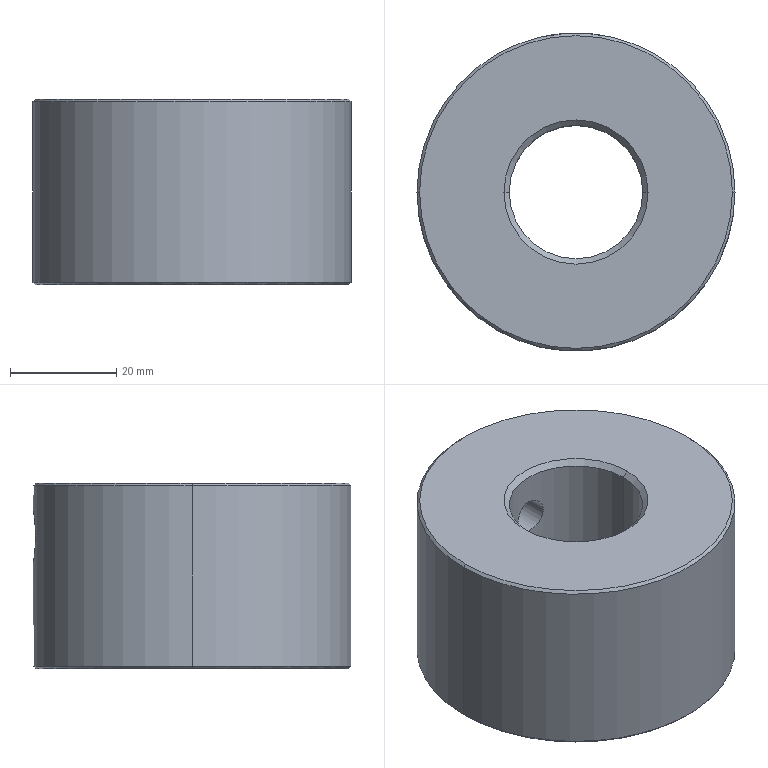Part | NX | 1 solid | 19 faces | box 60 x 60 x 35 mm | volume 80516 mm3 | cone 8 | cylinder 8 | plane 3 | commonest cylinder face diameters 6.8 x2 10 x2 25.2 x2 60 x2
STEP:
#1=CARTESIAN_POINT('',(29.5,0.,-5.));
#2=VERTEX_POINT('',#1);
#3=CARTESIAN_POINT('',(-29.5,0.,-5.));
#4=VERTEX_POINT('',#3);
#5=CARTESIAN_POINT('',(0.,0.,-5.));
#6=DIRECTION('',(0.,0.,1.));
#7=DIRECTION('',(1.,0.,0.));
#8=AXIS2_PLACEMENT_3D('',#5,#6,#7);
#9=CIRCLE('',#8,29.5);
#10=EDGE_CURVE('',#2,#4,#9,.T.);
#11=ORIENTED_EDGE('',*,*,#10,.F.);
#12=CARTESIAN_POINT('',(0.,0.,-5.));
#13=DIRECTION('',(0.,0.,1.));
#14=DIRECTION('',(1.,0.,0.));
#15=AXIS2_PLACEMENT_3D('',#12,#13,#14);
#16=CIRCLE('',#15,29.5);
#17=EDGE_CURVE('',#4,#2,#16,.T.);
#18=ORIENTED_EDGE('',*,*,#17,.F.);
#19=EDGE_LOOP('',(#11,#18));
#20=FACE_BOUND('',#19,.T.);
#21=CARTESIAN_POINT('',(13.6,0.,-5.));
#22=VERTEX_POINT('',#21);
#23=CARTESIAN_POINT('',(-13.6,0.,-5.));
#24=VERTEX_POINT('',#23);
#25=CARTESIAN_POINT('',(0.,0.,-5.));
#26=DIRECTION('',(0.,0.,1.));
#27=DIRECTION('',(1.,0.,0.));
#28=AXIS2_PLACEMENT_3D('',#25,#26,#27);
#29=CIRCLE('',#28,13.6);
#30=EDGE_CURVE('',#22,#24,#29,.T.);
#31=ORIENTED_EDGE('',*,*,#30,.T.);
#32=CARTESIAN_POINT('',(0.,0.,-5.));
#33=DIRECTION('',(0.,0.,1.));
#34=DIRECTION('',(1.,0.,0.));
#35=AXIS2_PLACEMENT_3D('',#32,#33,#34);
#36=CIRCLE('',#35,13.6);
#37=EDGE_CURVE('',#24,#22,#36,.T.);
#38=ORIENTED_EDGE('',*,*,#37,.T.);
#39=EDGE_LOOP('',(#31,#38));
#40=FACE_BOUND('',#39,.T.);
#41=CARTESIAN_POINT('',(0.,0.,-5.));
#42=DIRECTION('',(0.,0.,1.));
#43=DIRECTION('',(1.,0.,0.));
#44=AXIS2_PLACEMENT_3D('',#41,#42,#43);
#45=PLANE('',#44);
#46=ADVANCED_FACE('',(#20,#40),#45,.F.);
#47=CARTESIAN_POINT('',(12.6,0.,29.));
#48=VERTEX_POINT('',#47);
#49=CARTESIAN_POINT('',(-12.6,0.,29.));
#50=VERTEX_POINT('',#49);
#51=CARTESIAN_POINT('',(0.,0.,29.));
#52=DIRECTION('',(0.,0.,1.));
#53=DIRECTION('',(1.,0.,0.));
#54=AXIS2_PLACEMENT_3D('',#51,#52,#53);
#55=CIRCLE('',#54,12.6);
#56=EDGE_CURVE('',#48,#50,#55,.T.);
#57=ORIENTED_EDGE('',*,*,#56,.F.);
#58=CARTESIAN_POINT('',(13.6,0.,30.));
#59=VERTEX_POINT('',#58);
#60=CARTESIAN_POINT('',(13.1,0.,29.5));
#61=DIRECTION('',(0.7071,0.,0.7071));
#62=VECTOR('',#61,1000.);
#63=LINE('',#60,#62);
#64=EDGE_CURVE('',#48,#59,#63,.T.);
#65=ORIENTED_EDGE('',*,*,#64,.T.);
#66=CARTESIAN_POINT('',(-13.6,0.,30.));
#67=VERTEX_POINT('',#66);
#68=CARTESIAN_POINT('',(0.,0.,30.));
#69=DIRECTION('',(0.,0.,1.));
#70=DIRECTION('',(1.,0.,0.));
#71=AXIS2_PLACEMENT_3D('',#68,#69,#70);
#72=CIRCLE('',#71,13.6);
#73=EDGE_CURVE('',#59,#67,#72,.T.);
#74=ORIENTED_EDGE('',*,*,#73,.T.);
#75=CARTESIAN_POINT('',(-13.1,0.,29.5));
#76=DIRECTION('',(-0.7071,0.,0.7071));
#77=VECTOR('',#76,1000.);
#78=LINE('',#75,#77);
#79=EDGE_CURVE('',#50,#67,#78,.T.);
#80=ORIENTED_EDGE('',*,*,#79,.F.);
#81=EDGE_LOOP('',(#57,#65,#74,#80));
#82=FACE_BOUND('',#81,.T.);
#83=CARTESIAN_POINT('',(0.,0.,29.5));
#84=DIRECTION('',(0.,0.,1.));
#85=DIRECTION('',(1.,0.,0.));
#86=AXIS2_PLACEMENT_3D('',#83,#84,#85);
#87=CONICAL_SURFACE('',#86,13.1,0.7854);
#88=ADVANCED_FACE('',(#82),#87,.F.);
#89=CARTESIAN_POINT('',(-30.,0.,29.5));
#90=VERTEX_POINT('',#89);
#91=CARTESIAN_POINT('',(30.,0.,29.5));
#92=VERTEX_POINT('',#91);
#93=CARTESIAN_POINT('',(0.,0.,29.5));
#94=DIRECTION('',(0.,0.,-1.));
#95=DIRECTION('',(-1.,0.,0.));
#96=AXIS2_PLACEMENT_3D('',#93,#94,#95);
#97=CIRCLE('',#96,30.);
#98=EDGE_CURVE('',#90,#92,#97,.T.);
#99=ORIENTED_EDGE('',*,*,#98,.T.);
#100=CARTESIAN_POINT('',(30.,0.,-4.5));
#101=VERTEX_POINT('',#100);
#102=CARTESIAN_POINT('',(30.,0.,0.));
#103=DIRECTION('',(0.,0.,1.));
#104=VECTOR('',#103,1000.);
#105=LINE('',#102,#104);
#106=EDGE_CURVE('',#101,#92,#105,.T.);
#107=ORIENTED_EDGE('',*,*,#106,.F.);
#108=CARTESIAN_POINT('',(-30.,0.,-4.5));
#109=VERTEX_POINT('',#108);
#110=CARTESIAN_POINT('',(0.,0.,-4.5));
#111=DIRECTION('',(0.,0.,1.));
#112=DIRECTION('',(1.,0.,0.));
#113=AXIS2_PLACEMENT_3D('',#110,#111,#112);
#114=CIRCLE('',#113,30.);
#115=EDGE_CURVE('',#101,#109,#114,.T.);
#116=ORIENTED_EDGE('',*,*,#115,.T.);
#117=CARTESIAN_POINT('',(-30.,0.,0.));
#118=DIRECTION('',(0.,0.,1.));
#119=VECTOR('',#118,1000.);
#120=LINE('',#117,#119);
#121=EDGE_CURVE('',#109,#90,#120,.T.);
#122=ORIENTED_EDGE('',*,*,#121,.T.);
#123=EDGE_LOOP('',(#99,#107,#116,#122));
#124=FACE_BOUND('',#123,.T.);
#125=CARTESIAN_POINT('',(5.,29.58,20.));
#126=VERTEX_POINT('',#125);
#127=CARTESIAN_POINT('',(-5.,29.58,20.));
#128=VERTEX_POINT('',#127);
#129=CARTESIAN_POINT('',(-5.,29.58,20.));
#130=CARTESIAN_POINT('',(-5.,29.58,18.675));
#131=CARTESIAN_POINT('',(-3.919,29.792,16.092));
#132=CARTESIAN_POINT('',(0.0004669,30.104,14.454));
#133=CARTESIAN_POINT('',(3.917,29.792,16.091));
#134=CARTESIAN_POINT('',(5.,29.58,18.673));
#135=CARTESIAN_POINT('',(5.,29.58,20.));
#136=B_SPLINE_CURVE_WITH_KNOTS('',3,(#129,#130,#131,#132,#133,#134,#135),.UNSPECIFIED.,.F.,.F.,(4,1,1,1,4),(0.,0.25,0.5,0.75,1.),.UNSPECIFIED.);
#137=EDGE_CURVE('',#126,#128,#136,.F.);
#138=ORIENTED_EDGE('',*,*,#137,.F.);
#139=CARTESIAN_POINT('',(5.,29.58,20.));
#140=CARTESIAN_POINT('',(5.,29.58,21.269));
#141=CARTESIAN_POINT('',(3.919,29.792,23.936));
#142=CARTESIAN_POINT('',(0.00008607,30.104,25.533));
#143=CARTESIAN_POINT('',(-3.919,29.792,23.934));
#144=CARTESIAN_POINT('',(-5.,29.58,21.273));
#145=CARTESIAN_POINT('',(-5.,29.58,20.));
#146=B_SPLINE_CURVE_WITH_KNOTS('',3,(#139,#140,#141,#142,#143,#144,#145),.UNSPECIFIED.,.F.,.F.,(4,1,1,1,4),(0.,0.25,0.5,0.75,1.),.UNSPECIFIED.);
#147=EDGE_CURVE('',#128,#126,#146,.F.);
#148=ORIENTED_EDGE('',*,*,#147,.F.);
#149=EDGE_LOOP('',(#138,#148));
#150=FACE_BOUND('',#149,.T.);
#151=CARTESIAN_POINT('',(0.,0.,0.));
#152=DIRECTION('',(0.,0.,1.));
#153=DIRECTION('',(1.,0.,0.));
#154=AXIS2_PLACEMENT_3D('',#151,#152,#153);
#155=CYLINDRICAL_SURFACE('',#154,30.);
#156=ADVANCED_FACE('',(#124,#150),#155,.T.);
#157=CARTESIAN_POINT('',(29.5,0.,30.));
#158=VERTEX_POINT('',#157);
#159=CARTESIAN_POINT('',(-29.5,0.,30.));
#160=VERTEX_POINT('',#159);
#161=CARTESIAN_POINT('',(0.,0.,30.));
#162=DIRECTION('',(0.,0.,-1.));
#163=DIRECTION('',(-1.,0.,0.));
#164=AXIS2_PLACEMENT_3D('',#161,#162,#163);
#165=CIRCLE('',#164,29.5);
#166=EDGE_CURVE('',#158,#160,#165,.T.);
#167=ORIENTED_EDGE('',*,*,#166,.F.);
#168=CARTESIAN_POINT('',(0.,0.,30.));
#169=DIRECTION('',(0.,0.,-1.));
#170=DIRECTION('',(-1.,0.,0.));
#171=AXIS2_PLACEMENT_3D('',#168,#169,#170);
#172=CIRCLE('',#171,29.5);
#173=EDGE_CURVE('',#160,#158,#172,.T.);
#174=ORIENTED_EDGE('',*,*,#173,.F.);
#175=EDGE_LOOP('',(#167,#174));
#176=FACE_BOUND('',#175,.T.);
#177=CARTESIAN_POINT('',(0.,0.,30.));
#178=DIRECTION('',(0.,0.,1.));
#179=DIRECTION('',(1.,0.,0.));
#180=AXIS2_PLACEMENT_3D('',#177,#178,#179);
#181=CIRCLE('',#180,13.6);
#182=EDGE_CURVE('',#67,#59,#181,.T.);
#183=ORIENTED_EDGE('',*,*,#182,.F.);
#184=ORIENTED_EDGE('',*,*,#73,.F.);
#185=EDGE_LOOP('',(#183,#184));
#186=FACE_BOUND('',#185,.T.);
#187=CARTESIAN_POINT('',(0.,0.,30.));
#188=DIRECTION('',(0.,0.,1.));
#189=DIRECTION('',(1.,0.,0.));
#190=AXIS2_PLACEMENT_3D('',#187,#188,#189);
#191=PLANE('',#190);
#192=ADVANCED_FACE('',(#176,#186),#191,.T.);
#193=ORIENTED_EDGE('',*,*,#115,.F.);
#194=CARTESIAN_POINT('',(30.,0.,-4.5));
#195=DIRECTION('',(0.7071,0.,0.7071));
#196=VECTOR('',#195,1000.);
#197=LINE('',#194,#196);
#198=EDGE_CURVE('',#2,#101,#197,.T.);
#199=ORIENTED_EDGE('',*,*,#198,.F.);
#200=ORIENTED_EDGE('',*,*,#10,.T.);
#201=CARTESIAN_POINT('',(-30.,0.,-4.5));
#202=DIRECTION('',(-0.7071,0.,0.7071));
#203=VECTOR('',#202,1000.);
#204=LINE('',#201,#203);
#205=EDGE_CURVE('',#4,#109,#204,.T.);
#206=ORIENTED_EDGE('',*,*,#205,.T.);
#207=EDGE_LOOP('',(#193,#199,#200,#206));
#208=FACE_BOUND('',#207,.T.);
#209=CARTESIAN_POINT('',(0.,0.,-4.5));
#210=DIRECTION('',(0.,0.,1.));
#211=DIRECTION('',(1.,0.,0.));
#212=AXIS2_PLACEMENT_3D('',#209,#210,#211);
#213=CONICAL_SURFACE('',#212,30.,0.7854);
#214=ADVANCED_FACE('',(#208),#213,.T.);
#215=ORIENTED_EDGE('',*,*,#56,.T.);
#216=CARTESIAN_POINT('',(-12.6,0.,-4.));
#217=VERTEX_POINT('',#216);
#218=CARTESIAN_POINT('',(-12.6,0.,0.));
#219=DIRECTION('',(0.,0.,1.));
#220=VECTOR('',#219,1000.);
#221=LINE('',#218,#220);
#222=EDGE_CURVE('',#50,#217,#221,.F.);
#223=ORIENTED_EDGE('',*,*,#222,.T.);
#224=CARTESIAN_POINT('',(12.6,0.,-4.));
#225=VERTEX_POINT('',#224);
#226=CARTESIAN_POINT('',(0.,0.,-4.));
#227=DIRECTION('',(0.,0.,1.));
#228=DIRECTION('',(1.,0.,0.));
#229=AXIS2_PLACEMENT_3D('',#226,#227,#228);
#230=CIRCLE('',#229,12.6);
#231=EDGE_CURVE('',#225,#217,#230,.T.);
#232=ORIENTED_EDGE('',*,*,#231,.F.);
#233=CARTESIAN_POINT('',(12.6,0.,0.));
#234=DIRECTION('',(0.,0.,1.));
#235=VECTOR('',#234,1000.);
#236=LINE('',#233,#235);
#237=EDGE_CURVE('',#48,#225,#236,.F.);
#238=ORIENTED_EDGE('',*,*,#237,.F.);
#239=EDGE_LOOP('',(#215,#223,#232,#238));
#240=FACE_BOUND('',#239,.T.);
#241=CARTESIAN_POINT('',(-3.4,12.133,20.));
#242=VERTEX_POINT('',#241);
#243=CARTESIAN_POINT('',(3.4,12.133,20.));
#244=VERTEX_POINT('',#243);
#245=CARTESIAN_POINT('',(-3.4,12.133,20.));
#246=CARTESIAN_POINT('',(-3.4,12.133,20.9));
#247=CARTESIAN_POINT('',(-2.664,12.371,22.659));
#248=CARTESIAN_POINT('',(-0.00003224,12.715,23.771));
#249=CARTESIAN_POINT('',(2.664,12.371,22.658));
#250=CARTESIAN_POINT('',(3.4,12.133,20.901));
#251=CARTESIAN_POINT('',(3.4,12.133,20.));
#252=B_SPLINE_CURVE_WITH_KNOTS('',3,(#245,#246,#247,#248,#249,#250,#251),.UNSPECIFIED.,.F.,.F.,(4,1,1,1,4),(0.,0.25,0.5,0.75,1.),.UNSPECIFIED.);
#253=EDGE_CURVE('',#242,#244,#252,.T.);
#254=ORIENTED_EDGE('',*,*,#253,.T.);
#255=CARTESIAN_POINT('',(3.4,12.133,20.));
#256=CARTESIAN_POINT('',(3.4,12.133,19.1));
#257=CARTESIAN_POINT('',(2.664,12.371,17.341));
#258=CARTESIAN_POINT('',(0.00002958,12.715,16.229));
#259=CARTESIAN_POINT('',(-2.664,12.371,17.342));
#260=CARTESIAN_POINT('',(-3.4,12.133,19.099));
#261=CARTESIAN_POINT('',(-3.4,12.133,20.));
#262=B_SPLINE_CURVE_WITH_KNOTS('',3,(#255,#256,#257,#258,#259,#260,#261),.UNSPECIFIED.,.F.,.F.,(4,1,1,1,4),(0.,0.25,0.5,0.75,1.),.UNSPECIFIED.);
#263=EDGE_CURVE('',#244,#242,#262,.T.);
#264=ORIENTED_EDGE('',*,*,#263,.T.);
#265=EDGE_LOOP('',(#254,#264));
#266=FACE_BOUND('',#265,.T.);
#267=CARTESIAN_POINT('',(0.,0.,0.));
#268=DIRECTION('',(0.,0.,1.));
#269=DIRECTION('',(1.,0.,0.));
#270=AXIS2_PLACEMENT_3D('',#267,#268,#269);
#271=CYLINDRICAL_SURFACE('',#270,12.6);
#272=ADVANCED_FACE('',(#240,#266),#271,.F.);
#273=CARTESIAN_POINT('',(-3.4,24.5,20.));
#274=VERTEX_POINT('',#273);
#275=CARTESIAN_POINT('',(3.4,24.5,20.));
#276=VERTEX_POINT('',#275);
#277=CARTESIAN_POINT('',(0.,24.5,20.));
#278=DIRECTION('',(0.,1.,0.));
#279=DIRECTION('',(1.,0.,0.));
#280=AXIS2_PLACEMENT_3D('',#277,#278,#279);
#281=CIRCLE('',#280,3.4);
#282=EDGE_CURVE('',#274,#276,#281,.T.);
#283=ORIENTED_EDGE('',*,*,#282,.T.);
#284=CARTESIAN_POINT('',(3.4,30.,20.));
#285=DIRECTION('',(0.,1.,0.));
#286=VECTOR('',#285,1000.);
#287=LINE('',#284,#286);
#288=EDGE_CURVE('',#244,#276,#287,.T.);
#289=ORIENTED_EDGE('',*,*,#288,.F.);
#290=ORIENTED_EDGE('',*,*,#253,.F.);
#291=CARTESIAN_POINT('',(-3.4,30.,20.));
#292=DIRECTION('',(0.,1.,0.));
#293=VECTOR('',#292,1000.);
#294=LINE('',#291,#293);
#295=EDGE_CURVE('',#242,#274,#294,.T.);
#296=ORIENTED_EDGE('',*,*,#295,.T.);
#297=EDGE_LOOP('',(#283,#289,#290,#296));
#298=FACE_BOUND('',#297,.T.);
#299=CARTESIAN_POINT('',(0.,30.,20.));
#300=DIRECTION('',(0.,1.,0.));
#301=DIRECTION('',(1.,0.,0.));
#302=AXIS2_PLACEMENT_3D('',#299,#300,#301);
#303=CYLINDRICAL_SURFACE('',#302,3.4);
#304=ADVANCED_FACE('',(#298),#303,.F.);
#305=CARTESIAN_POINT('',(5.,24.5,20.));
#306=VERTEX_POINT('',#305);
#307=CARTESIAN_POINT('',(-5.,24.5,20.));
#308=VERTEX_POINT('',#307);
#309=CARTESIAN_POINT('',(0.,24.5,20.));
#310=DIRECTION('',(0.,1.,0.));
#311=DIRECTION('',(-1.,0.,0.));
#312=AXIS2_PLACEMENT_3D('',#309,#310,#311);
#313=CIRCLE('',#312,5.);
#314=EDGE_CURVE('',#306,#308,#313,.T.);
#315=ORIENTED_EDGE('',*,*,#314,.T.);
#316=CARTESIAN_POINT('',(0.,24.5,20.));
#317=DIRECTION('',(0.,1.,0.));
#318=DIRECTION('',(-1.,0.,0.));
#319=AXIS2_PLACEMENT_3D('',#316,#317,#318);
#320=CIRCLE('',#319,5.);
#321=EDGE_CURVE('',#308,#306,#320,.T.);
#322=ORIENTED_EDGE('',*,*,#321,.T.);
#323=EDGE_LOOP('',(#315,#322));
#324=FACE_BOUND('',#323,.T.);
#325=ORIENTED_EDGE('',*,*,#282,.F.);
#326=CARTESIAN_POINT('',(0.,24.5,20.));
#327=DIRECTION('',(0.,1.,0.));
#328=DIRECTION('',(1.,0.,0.));
#329=AXIS2_PLACEMENT_3D('',#326,#327,#328);
#330=CIRCLE('',#329,3.4);
#331=EDGE_CURVE('',#276,#274,#330,.T.);
#332=ORIENTED_EDGE('',*,*,#331,.F.);
#333=EDGE_LOOP('',(#325,#332));
#334=FACE_BOUND('',#333,.T.);
#335=CARTESIAN_POINT('',(-332.038,24.5,-73.917));
#336=DIRECTION('',(0.,1.,0.));
#337=DIRECTION('',(1.,0.,0.));
#338=AXIS2_PLACEMENT_3D('',#335,#336,#337);
#339=PLANE('',#338);
#340=ADVANCED_FACE('',(#324,#334),#339,.T.);
#341=ORIENTED_EDGE('',*,*,#314,.F.);
#342=CARTESIAN_POINT('',(5.,38.5,20.));
#343=DIRECTION('',(0.,1.,0.));
#344=VECTOR('',#343,1000.);
#345=LINE('',#342,#344);
#346=EDGE_CURVE('',#126,#306,#345,.F.);
#347=ORIENTED_EDGE('',*,*,#346,.F.);
#348=ORIENTED_EDGE('',*,*,#137,.T.);
#349=CARTESIAN_POINT('',(-5.,38.5,20.));
#350=DIRECTION('',(0.,1.,0.));
#351=VECTOR('',#350,1000.);
#352=LINE('',#349,#351);
#353=EDGE_CURVE('',#128,#308,#352,.F.);
#354=ORIENTED_EDGE('',*,*,#353,.T.);
#355=EDGE_LOOP('',(#341,#347,#348,#354));
#356=FACE_BOUND('',#355,.T.);
#357=CARTESIAN_POINT('',(0.,38.5,20.));
#358=DIRECTION('',(0.,1.,0.));
#359=DIRECTION('',(-1.,0.,0.));
#360=AXIS2_PLACEMENT_3D('',#357,#358,#359);
#361=CYLINDRICAL_SURFACE('',#360,5.);
#362=ADVANCED_FACE('',(#356),#361,.F.);
#363=ORIENTED_EDGE('',*,*,#98,.F.);
#364=CARTESIAN_POINT('',(-29.5,0.,30.));
#365=DIRECTION('',(-0.7071,0.,-0.7071));
#366=VECTOR('',#365,1000.);
#367=LINE('',#364,#366);
#368=EDGE_CURVE('',#90,#160,#367,.F.);
#369=ORIENTED_EDGE('',*,*,#368,.T.);
#370=ORIENTED_EDGE('',*,*,#173,.T.);
#371=CARTESIAN_POINT('',(29.5,0.,30.));
#372=DIRECTION('',(0.7071,0.,-0.7071));
#373=VECTOR('',#372,1000.);
#374=LINE('',#371,#373);
#375=EDGE_CURVE('',#92,#158,#374,.F.);
#376=ORIENTED_EDGE('',*,*,#375,.F.);
#377=EDGE_LOOP('',(#363,#369,#370,#376));
#378=FACE_BOUND('',#377,.T.);
#379=CARTESIAN_POINT('',(0.,0.,30.));
#380=DIRECTION('',(0.,0.,-1.));
#381=DIRECTION('',(-1.,0.,0.));
#382=AXIS2_PLACEMENT_3D('',#379,#380,#381);
#383=CONICAL_SURFACE('',#382,29.5,0.7854);
#384=ADVANCED_FACE('',(#378),#383,.T.);
#385=CARTESIAN_POINT('',(0.,0.,-4.));
#386=DIRECTION('',(0.,0.,1.));
#387=DIRECTION('',(1.,0.,0.));
#388=AXIS2_PLACEMENT_3D('',#385,#386,#387);
#389=CIRCLE('',#388,12.6);
#390=EDGE_CURVE('',#217,#225,#389,.T.);
#391=ORIENTED_EDGE('',*,*,#390,.T.);
#392=CARTESIAN_POINT('',(13.6,0.,-5.));
#393=DIRECTION('',(0.7071,0.,-0.7071));
#394=VECTOR('',#393,1000.);
#395=LINE('',#392,#394);
#396=EDGE_CURVE('',#225,#22,#395,.T.);
#397=ORIENTED_EDGE('',*,*,#396,.T.);
#398=ORIENTED_EDGE('',*,*,#37,.F.);
#399=CARTESIAN_POINT('',(-13.6,0.,-5.));
#400=DIRECTION('',(-0.7071,0.,-0.7071));
#401=VECTOR('',#400,1000.);
#402=LINE('',#399,#401);
#403=EDGE_CURVE('',#217,#24,#402,.T.);
#404=ORIENTED_EDGE('',*,*,#403,.F.);
#405=EDGE_LOOP('',(#391,#397,#398,#404));
#406=FACE_BOUND('',#405,.T.);
#407=CARTESIAN_POINT('',(0.,0.,-5.));
#408=DIRECTION('',(0.,0.,-1.));
#409=DIRECTION('',(-1.,0.,0.));
#410=AXIS2_PLACEMENT_3D('',#407,#408,#409);
#411=CONICAL_SURFACE('',#410,13.6,0.7854);
#412=ADVANCED_FACE('',(#406),#411,.F.);
#413=ORIENTED_EDGE('',*,*,#166,.T.);
#414=ORIENTED_EDGE('',*,*,#368,.F.);
#415=CARTESIAN_POINT('',(0.,0.,29.5));
#416=DIRECTION('',(0.,0.,-1.));
#417=DIRECTION('',(-1.,0.,0.));
#418=AXIS2_PLACEMENT_3D('',#415,#416,#417);
#419=CIRCLE('',#418,30.);
#420=EDGE_CURVE('',#92,#90,#419,.T.);
#421=ORIENTED_EDGE('',*,*,#420,.F.);
#422=ORIENTED_EDGE('',*,*,#375,.T.);
#423=EDGE_LOOP('',(#413,#414,#421,#422));
#424=FACE_BOUND('',#423,.T.);
#425=CARTESIAN_POINT('',(0.,0.,30.));
#426=DIRECTION('',(0.,0.,-1.));
#427=DIRECTION('',(-1.,0.,0.));
#428=AXIS2_PLACEMENT_3D('',#425,#426,#427);
#429=CONICAL_SURFACE('',#428,29.5,0.7854);
#430=ADVANCED_FACE('',(#424),#429,.T.);
#431=ORIENTED_EDGE('',*,*,#198,.T.);
#432=CARTESIAN_POINT('',(0.,0.,-4.5));
#433=DIRECTION('',(0.,0.,1.));
#434=DIRECTION('',(1.,0.,0.));
#435=AXIS2_PLACEMENT_3D('',#432,#433,#434);
#436=CIRCLE('',#435,30.);
#437=EDGE_CURVE('',#109,#101,#436,.T.);
#438=ORIENTED_EDGE('',*,*,#437,.F.);
#439=ORIENTED_EDGE('',*,*,#205,.F.);
#440=ORIENTED_EDGE('',*,*,#17,.T.);
#441=EDGE_LOOP('',(#431,#438,#439,#440));
#442=FACE_BOUND('',#441,.T.);
#443=CARTESIAN_POINT('',(0.,0.,-4.5));
#444=DIRECTION('',(0.,0.,1.));
#445=DIRECTION('',(1.,0.,0.));
#446=AXIS2_PLACEMENT_3D('',#443,#444,#445);
#447=CONICAL_SURFACE('',#446,30.,0.7854);
#448=ADVANCED_FACE('',(#442),#447,.T.);
#449=ORIENTED_EDGE('',*,*,#288,.T.);
#450=ORIENTED_EDGE('',*,*,#331,.T.);
#451=ORIENTED_EDGE('',*,*,#295,.F.);
#452=ORIENTED_EDGE('',*,*,#263,.F.);
#453=EDGE_LOOP('',(#449,#450,#451,#452));
#454=FACE_BOUND('',#453,.T.);
#455=CARTESIAN_POINT('',(0.,30.,20.));
#456=DIRECTION('',(0.,1.,0.));
#457=DIRECTION('',(1.,0.,0.));
#458=AXIS2_PLACEMENT_3D('',#455,#456,#457);
#459=CYLINDRICAL_SURFACE('',#458,3.4);
#460=ADVANCED_FACE('',(#454),#459,.F.);
#461=ORIENTED_EDGE('',*,*,#182,.T.);
#462=ORIENTED_EDGE('',*,*,#64,.F.);
#463=CARTESIAN_POINT('',(0.,0.,29.));
#464=DIRECTION('',(0.,0.,1.));
#465=DIRECTION('',(1.,0.,0.));
#466=AXIS2_PLACEMENT_3D('',#463,#464,#465);
#467=CIRCLE('',#466,12.6);
#468=EDGE_CURVE('',#50,#48,#467,.T.);
#469=ORIENTED_EDGE('',*,*,#468,.F.);
#470=ORIENTED_EDGE('',*,*,#79,.T.);
#471=EDGE_LOOP('',(#461,#462,#469,#470));
#472=FACE_BOUND('',#471,.T.);
#473=CARTESIAN_POINT('',(0.,0.,29.5));
#474=DIRECTION('',(0.,0.,1.));
#475=DIRECTION('',(1.,0.,0.));
#476=AXIS2_PLACEMENT_3D('',#473,#474,#475);
#477=CONICAL_SURFACE('',#476,13.1,0.7854);
#478=ADVANCED_FACE('',(#472),#477,.F.);
#479=ORIENTED_EDGE('',*,*,#390,.F.);
#480=ORIENTED_EDGE('',*,*,#222,.F.);
#481=ORIENTED_EDGE('',*,*,#468,.T.);
#482=ORIENTED_EDGE('',*,*,#237,.T.);
#483=EDGE_LOOP('',(#479,#480,#481,#482));
#484=FACE_BOUND('',#483,.T.);
#485=CARTESIAN_POINT('',(0.,0.,0.));
#486=DIRECTION('',(0.,0.,1.));
#487=DIRECTION('',(1.,0.,0.));
#488=AXIS2_PLACEMENT_3D('',#485,#486,#487);
#489=CYLINDRICAL_SURFACE('',#488,12.6);
#490=ADVANCED_FACE('',(#484),#489,.F.);
#491=ORIENTED_EDGE('',*,*,#30,.F.);
#492=ORIENTED_EDGE('',*,*,#396,.F.);
#493=ORIENTED_EDGE('',*,*,#231,.T.);
#494=ORIENTED_EDGE('',*,*,#403,.T.);
#495=EDGE_LOOP('',(#491,#492,#493,#494));
#496=FACE_BOUND('',#495,.T.);
#497=CARTESIAN_POINT('',(0.,0.,-5.));
#498=DIRECTION('',(0.,0.,-1.));
#499=DIRECTION('',(-1.,0.,0.));
#500=AXIS2_PLACEMENT_3D('',#497,#498,#499);
#501=CONICAL_SURFACE('',#500,13.6,0.7854);
#502=ADVANCED_FACE('',(#496),#501,.F.);
#503=ORIENTED_EDGE('',*,*,#353,.F.);
#504=ORIENTED_EDGE('',*,*,#147,.T.);
#505=ORIENTED_EDGE('',*,*,#346,.T.);
#506=ORIENTED_EDGE('',*,*,#321,.F.);
#507=EDGE_LOOP('',(#503,#504,#505,#506));
#508=FACE_BOUND('',#507,.T.);
#509=CARTESIAN_POINT('',(0.,38.5,20.));
#510=DIRECTION('',(0.,1.,0.));
#511=DIRECTION('',(-1.,0.,0.));
#512=AXIS2_PLACEMENT_3D('',#509,#510,#511);
#513=CYLINDRICAL_SURFACE('',#512,5.);
#514=ADVANCED_FACE('',(#508),#513,.F.);
#515=ORIENTED_EDGE('',*,*,#106,.T.);
#516=ORIENTED_EDGE('',*,*,#420,.T.);
#517=ORIENTED_EDGE('',*,*,#121,.F.);
#518=ORIENTED_EDGE('',*,*,#437,.T.);
#519=EDGE_LOOP('',(#515,#516,#517,#518));
#520=FACE_BOUND('',#519,.T.);
#521=CARTESIAN_POINT('',(0.,0.,0.));
#522=DIRECTION('',(0.,0.,1.));
#523=DIRECTION('',(1.,0.,0.));
#524=AXIS2_PLACEMENT_3D('',#521,#522,#523);
#525=CYLINDRICAL_SURFACE('',#524,30.);
#526=ADVANCED_FACE('',(#520),#525,.T.);
#527=CLOSED_SHELL('',(#46,#88,#156,#192,#214,#272,#304,#340,#362,#384,#412,#430,#448,#460,#478,#490,#502,#514,#526));
#528=MANIFOLD_SOLID_BREP('',#527);
#529=(LENGTH_UNIT()NAMED_UNIT(*)SI_UNIT(.MILLI.,.METRE.));
#530=UNCERTAINTY_MEASURE_WITH_UNIT(LENGTH_MEASURE(0.0508),#529,'','');
#531=(NAMED_UNIT(*)PLANE_ANGLE_UNIT()SI_UNIT($,.RADIAN.));
#532=(NAMED_UNIT(*)SI_UNIT($,.STERADIAN.)SOLID_ANGLE_UNIT());
#533=(GEOMETRIC_REPRESENTATION_CONTEXT(3)GLOBAL_UNCERTAINTY_ASSIGNED_CONTEXT((#530))GLOBAL_UNIT_ASSIGNED_CONTEXT((#529,#531,#532))REPRESENTATION_CONTEXT('',''));
#534=ADVANCED_BREP_SHAPE_REPRESENTATION('',(#528),#533);